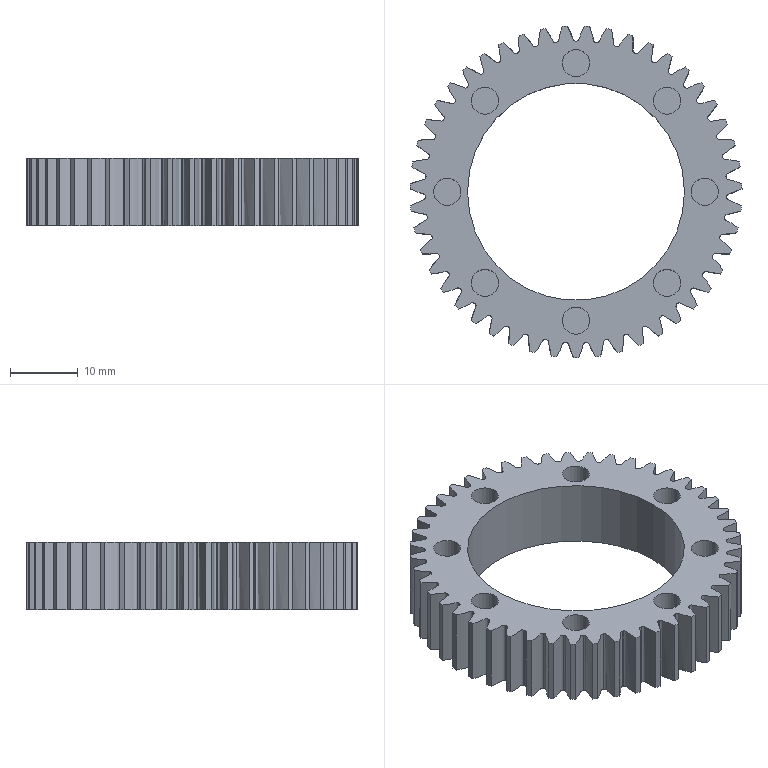Part | SolidWorks | features ICE 3, CirPattern 1, Extrusion 1, RefAxis 1 | 1 solid | 216 faces | box 48.992 x 48.968 x 10 mm | volume 8395 mm3 | cylinder 112 | spline 94 | plane 10 | commonest cylinder face diameters 44.5 x47 49 x47 4 x16 32 x2